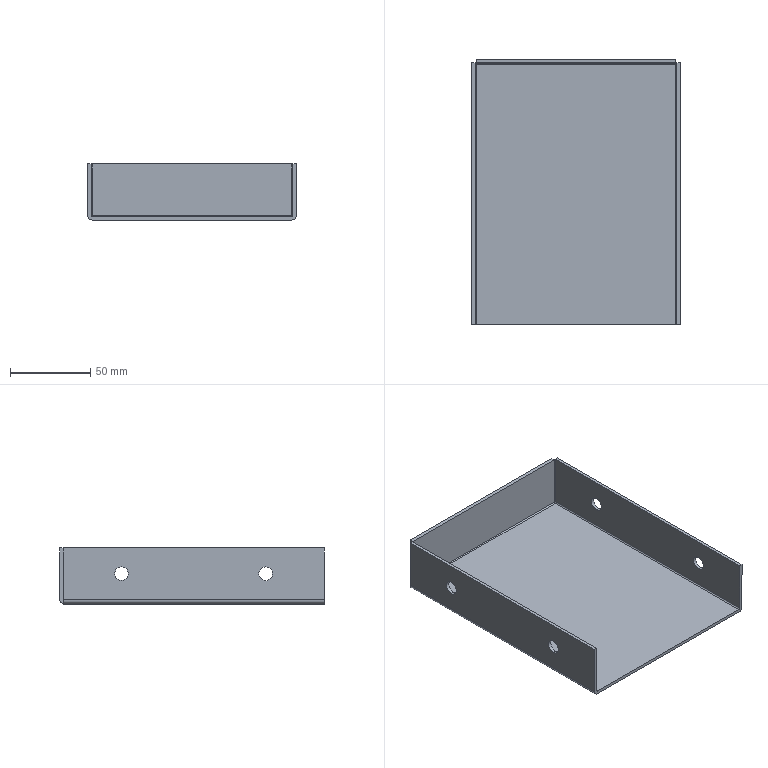Part | SolidWorks | features BaseBody 1 | 1 solid | 32 faces | box 130 x 165 x 35 mm | volume 71487 mm3 | plane 18 | cylinder 14 | commonest cylinder face diameters 8.5 x8 1.473 x3 5.473 x3
STEP:
#1=CARTESIAN_POINT('',(65.,45.,21.118));
#2=VERTEX_POINT('',#1);
#3=CARTESIAN_POINT('',(65.,45.,12.618));
#4=VERTEX_POINT('',#3);
#5=CARTESIAN_POINT('',(65.,45.,16.868));
#6=DIRECTION('',(1.,0.,0.));
#7=DIRECTION('',(0.,0.,1.));
#8=AXIS2_PLACEMENT_3D('',#5,#6,#7);
#9=CIRCLE('',#8,4.25);
#10=EDGE_CURVE('',#2,#4,#9,.T.);
#11=ORIENTED_EDGE('',*,*,#10,.T.);
#12=CARTESIAN_POINT('',(63.,45.,12.618));
#13=VERTEX_POINT('',#12);
#14=CARTESIAN_POINT('',(118.,45.,12.618));
#15=DIRECTION('',(-1.,0.,0.));
#16=VECTOR('',#15,1000.);
#17=LINE('',#14,#16);
#18=EDGE_CURVE('',#4,#13,#17,.T.);
#19=ORIENTED_EDGE('',*,*,#18,.T.);
#20=CARTESIAN_POINT('',(63.,45.,21.118));
#21=VERTEX_POINT('',#20);
#22=CARTESIAN_POINT('',(63.,45.,16.868));
#23=DIRECTION('',(1.,0.,0.));
#24=DIRECTION('',(0.,0.,1.));
#25=AXIS2_PLACEMENT_3D('',#22,#23,#24);
#26=CIRCLE('',#25,4.25);
#27=EDGE_CURVE('',#21,#13,#26,.T.);
#28=ORIENTED_EDGE('',*,*,#27,.F.);
#29=CARTESIAN_POINT('',(118.,45.,21.118));
#30=DIRECTION('',(-1.,0.,0.));
#31=VECTOR('',#30,1000.);
#32=LINE('',#29,#31);
#33=EDGE_CURVE('',#2,#21,#32,.T.);
#34=ORIENTED_EDGE('',*,*,#33,.F.);
#35=EDGE_LOOP('',(#11,#19,#28,#34));
#36=FACE_OUTER_BOUND('',#35,.T.);
#37=CARTESIAN_POINT('',(118.,45.,16.868));
#38=DIRECTION('',(-1.,0.,0.));
#39=DIRECTION('',(0.,0.,1.));
#40=AXIS2_PLACEMENT_3D('',#37,#38,#39);
#41=CYLINDRICAL_SURFACE('',#40,4.25);
#42=ADVANCED_FACE('',(#36),#41,.F.);
#43=CARTESIAN_POINT('',(65.,-45.,21.118));
#44=VERTEX_POINT('',#43);
#45=CARTESIAN_POINT('',(65.,-45.,12.618));
#46=VERTEX_POINT('',#45);
#47=CARTESIAN_POINT('',(65.,-45.,16.868));
#48=DIRECTION('',(1.,0.,0.));
#49=DIRECTION('',(0.,0.,1.));
#50=AXIS2_PLACEMENT_3D('',#47,#48,#49);
#51=CIRCLE('',#50,4.25);
#52=EDGE_CURVE('',#44,#46,#51,.T.);
#53=ORIENTED_EDGE('',*,*,#52,.T.);
#54=CARTESIAN_POINT('',(63.,-45.,12.618));
#55=VERTEX_POINT('',#54);
#56=CARTESIAN_POINT('',(118.,-45.,12.618));
#57=DIRECTION('',(-1.,0.,0.));
#58=VECTOR('',#57,1000.);
#59=LINE('',#56,#58);
#60=EDGE_CURVE('',#46,#55,#59,.T.);
#61=ORIENTED_EDGE('',*,*,#60,.T.);
#62=CARTESIAN_POINT('',(63.,-45.,21.118));
#63=VERTEX_POINT('',#62);
#64=CARTESIAN_POINT('',(63.,-45.,16.868));
#65=DIRECTION('',(1.,0.,0.));
#66=DIRECTION('',(0.,0.,1.));
#67=AXIS2_PLACEMENT_3D('',#64,#65,#66);
#68=CIRCLE('',#67,4.25);
#69=EDGE_CURVE('',#63,#55,#68,.T.);
#70=ORIENTED_EDGE('',*,*,#69,.F.);
#71=CARTESIAN_POINT('',(118.,-45.,21.118));
#72=DIRECTION('',(-1.,0.,0.));
#73=VECTOR('',#72,1000.);
#74=LINE('',#71,#73);
#75=EDGE_CURVE('',#44,#63,#74,.T.);
#76=ORIENTED_EDGE('',*,*,#75,.F.);
#77=EDGE_LOOP('',(#53,#61,#70,#76));
#78=FACE_OUTER_BOUND('',#77,.T.);
#79=CARTESIAN_POINT('',(118.,-45.,16.868));
#80=DIRECTION('',(-1.,0.,0.));
#81=DIRECTION('',(0.,0.,1.));
#82=AXIS2_PLACEMENT_3D('',#79,#80,#81);
#83=CYLINDRICAL_SURFACE('',#82,4.25);
#84=ADVANCED_FACE('',(#78),#83,.F.);
#85=CARTESIAN_POINT('',(-63.,45.,12.618));
#86=VERTEX_POINT('',#85);
#87=CARTESIAN_POINT('',(-63.,45.,21.118));
#88=VERTEX_POINT('',#87);
#89=CARTESIAN_POINT('',(-63.,45.,16.868));
#90=DIRECTION('',(-1.,0.,0.));
#91=DIRECTION('',(0.,0.,1.));
#92=AXIS2_PLACEMENT_3D('',#89,#90,#91);
#93=CIRCLE('',#92,4.25);
#94=EDGE_CURVE('',#86,#88,#93,.T.);
#95=ORIENTED_EDGE('',*,*,#94,.F.);
#96=CARTESIAN_POINT('',(-65.,45.,12.618));
#97=VERTEX_POINT('',#96);
#98=CARTESIAN_POINT('',(118.,45.,12.618));
#99=DIRECTION('',(-1.,0.,0.));
#100=VECTOR('',#99,1000.);
#101=LINE('',#98,#100);
#102=EDGE_CURVE('',#86,#97,#101,.T.);
#103=ORIENTED_EDGE('',*,*,#102,.T.);
#104=CARTESIAN_POINT('',(-65.,45.,21.118));
#105=VERTEX_POINT('',#104);
#106=CARTESIAN_POINT('',(-65.,45.,16.868));
#107=DIRECTION('',(-1.,0.,0.));
#108=DIRECTION('',(0.,0.,1.));
#109=AXIS2_PLACEMENT_3D('',#106,#107,#108);
#110=CIRCLE('',#109,4.25);
#111=EDGE_CURVE('',#97,#105,#110,.T.);
#112=ORIENTED_EDGE('',*,*,#111,.T.);
#113=CARTESIAN_POINT('',(118.,45.,21.118));
#114=DIRECTION('',(-1.,0.,0.));
#115=VECTOR('',#114,1000.);
#116=LINE('',#113,#115);
#117=EDGE_CURVE('',#88,#105,#116,.T.);
#118=ORIENTED_EDGE('',*,*,#117,.F.);
#119=EDGE_LOOP('',(#95,#103,#112,#118));
#120=FACE_OUTER_BOUND('',#119,.T.);
#121=CARTESIAN_POINT('',(118.,45.,16.868));
#122=DIRECTION('',(-1.,0.,0.));
#123=DIRECTION('',(0.,0.,1.));
#124=AXIS2_PLACEMENT_3D('',#121,#122,#123);
#125=CYLINDRICAL_SURFACE('',#124,4.25);
#126=ADVANCED_FACE('',(#120),#125,.F.);
#127=CARTESIAN_POINT('',(-63.,-45.,12.618));
#128=VERTEX_POINT('',#127);
#129=CARTESIAN_POINT('',(-63.,-45.,21.118));
#130=VERTEX_POINT('',#129);
#131=CARTESIAN_POINT('',(-63.,-45.,16.868));
#132=DIRECTION('',(-1.,0.,0.));
#133=DIRECTION('',(0.,0.,1.));
#134=AXIS2_PLACEMENT_3D('',#131,#132,#133);
#135=CIRCLE('',#134,4.25);
#136=EDGE_CURVE('',#128,#130,#135,.T.);
#137=ORIENTED_EDGE('',*,*,#136,.F.);
#138=CARTESIAN_POINT('',(-65.,-45.,12.618));
#139=VERTEX_POINT('',#138);
#140=CARTESIAN_POINT('',(118.,-45.,12.618));
#141=DIRECTION('',(-1.,0.,0.));
#142=VECTOR('',#141,1000.);
#143=LINE('',#140,#142);
#144=EDGE_CURVE('',#128,#139,#143,.T.);
#145=ORIENTED_EDGE('',*,*,#144,.T.);
#146=CARTESIAN_POINT('',(-65.,-45.,21.118));
#147=VERTEX_POINT('',#146);
#148=CARTESIAN_POINT('',(-65.,-45.,16.868));
#149=DIRECTION('',(-1.,0.,0.));
#150=DIRECTION('',(0.,0.,1.));
#151=AXIS2_PLACEMENT_3D('',#148,#149,#150);
#152=CIRCLE('',#151,4.25);
#153=EDGE_CURVE('',#139,#147,#152,.T.);
#154=ORIENTED_EDGE('',*,*,#153,.T.);
#155=CARTESIAN_POINT('',(118.,-45.,21.118));
#156=DIRECTION('',(-1.,0.,0.));
#157=VECTOR('',#156,1000.);
#158=LINE('',#155,#157);
#159=EDGE_CURVE('',#130,#147,#158,.T.);
#160=ORIENTED_EDGE('',*,*,#159,.F.);
#161=EDGE_LOOP('',(#137,#145,#154,#160));
#162=FACE_OUTER_BOUND('',#161,.T.);
#163=CARTESIAN_POINT('',(118.,-45.,16.868));
#164=DIRECTION('',(-1.,0.,0.));
#165=DIRECTION('',(0.,0.,1.));
#166=AXIS2_PLACEMENT_3D('',#163,#164,#165);
#167=CYLINDRICAL_SURFACE('',#166,4.25);
#168=ADVANCED_FACE('',(#162),#167,.F.);
#169=CARTESIAN_POINT('',(62.263,80.763,-2.));
#170=VERTEX_POINT('',#169);
#171=CARTESIAN_POINT('',(62.263,-81.5,-2.));
#172=VERTEX_POINT('',#171);
#173=CARTESIAN_POINT('',(62.263,0.,-2.));
#174=DIRECTION('',(0.,-1.,0.));
#175=VECTOR('',#174,1000.);
#176=LINE('',#173,#175);
#177=EDGE_CURVE('',#170,#172,#176,.T.);
#178=ORIENTED_EDGE('',*,*,#177,.T.);
#179=CARTESIAN_POINT('',(-62.263,-81.5,-2.));
#180=VERTEX_POINT('',#179);
#181=CARTESIAN_POINT('',(0.,-81.5,-2.));
#182=DIRECTION('',(-1.,0.,0.));
#183=VECTOR('',#182,1000.);
#184=LINE('',#181,#183);
#185=EDGE_CURVE('',#172,#180,#184,.T.);
#186=ORIENTED_EDGE('',*,*,#185,.T.);
#187=CARTESIAN_POINT('',(-62.263,80.763,-2.));
#188=VERTEX_POINT('',#187);
#189=CARTESIAN_POINT('',(-62.263,0.,-2.));
#190=DIRECTION('',(0.,1.,0.));
#191=VECTOR('',#190,1000.);
#192=LINE('',#189,#191);
#193=EDGE_CURVE('',#180,#188,#192,.T.);
#194=ORIENTED_EDGE('',*,*,#193,.T.);
#195=CARTESIAN_POINT('',(0.,80.763,-2.));
#196=DIRECTION('',(1.,0.,0.));
#197=VECTOR('',#196,1000.);
#198=LINE('',#195,#197);
#199=EDGE_CURVE('',#188,#170,#198,.T.);
#200=ORIENTED_EDGE('',*,*,#199,.T.);
#201=EDGE_LOOP('',(#178,#186,#194,#200));
#202=FACE_OUTER_BOUND('',#201,.T.);
#203=CARTESIAN_POINT('',(0.,0.,-2.));
#204=DIRECTION('',(0.,0.,-1.));
#205=DIRECTION('',(-1.,0.,0.));
#206=AXIS2_PLACEMENT_3D('',#203,#204,#205);
#207=PLANE('',#206);
#208=ADVANCED_FACE('',(#202),#207,.T.);
#209=ORIENTED_EDGE('',*,*,#185,.F.);
#210=CARTESIAN_POINT('',(65.,-81.5,0.7366));
#211=VERTEX_POINT('',#210);
#212=CARTESIAN_POINT('',(62.263,-81.5,0.7366));
#213=DIRECTION('',(0.,1.,0.));
#214=DIRECTION('',(0.,0.,1.));
#215=AXIS2_PLACEMENT_3D('',#212,#213,#214);
#216=CIRCLE('',#215,2.737);
#217=EDGE_CURVE('',#211,#172,#216,.T.);
#218=ORIENTED_EDGE('',*,*,#217,.F.);
#219=CARTESIAN_POINT('',(65.,-81.5,33.));
#220=VERTEX_POINT('',#219);
#221=CARTESIAN_POINT('',(65.,-81.5,0.));
#222=DIRECTION('',(0.,0.,1.));
#223=VECTOR('',#222,1000.);
#224=LINE('',#221,#223);
#225=EDGE_CURVE('',#211,#220,#224,.T.);
#226=ORIENTED_EDGE('',*,*,#225,.T.);
#227=CARTESIAN_POINT('',(63.,-81.5,33.));
#228=VERTEX_POINT('',#227);
#229=CARTESIAN_POINT('',(65.,-81.5,33.));
#230=DIRECTION('',(1.,0.,0.));
#231=VECTOR('',#230,1000.);
#232=LINE('',#229,#231);
#233=EDGE_CURVE('',#228,#220,#232,.T.);
#234=ORIENTED_EDGE('',*,*,#233,.F.);
#235=CARTESIAN_POINT('',(63.,-81.5,0.7366));
#236=VERTEX_POINT('',#235);
#237=CARTESIAN_POINT('',(63.,-81.5,0.));
#238=DIRECTION('',(0.,0.,1.));
#239=VECTOR('',#238,1000.);
#240=LINE('',#237,#239);
#241=EDGE_CURVE('',#236,#228,#240,.T.);
#242=ORIENTED_EDGE('',*,*,#241,.F.);
#243=CARTESIAN_POINT('',(62.263,-81.5,0.));
#244=VERTEX_POINT('',#243);
#245=CARTESIAN_POINT('',(62.263,-81.5,0.7366));
#246=DIRECTION('',(0.,1.,0.));
#247=DIRECTION('',(0.,0.,1.));
#248=AXIS2_PLACEMENT_3D('',#245,#246,#247);
#249=CIRCLE('',#248,0.7366);
#250=EDGE_CURVE('',#236,#244,#249,.T.);
#251=ORIENTED_EDGE('',*,*,#250,.T.);
#252=CARTESIAN_POINT('',(-62.263,-81.5,0.));
#253=VERTEX_POINT('',#252);
#254=CARTESIAN_POINT('',(-65.,-81.5,0.));
#255=DIRECTION('',(-1.,0.,0.));
#256=VECTOR('',#255,1000.);
#257=LINE('',#254,#256);
#258=EDGE_CURVE('',#244,#253,#257,.T.);
#259=ORIENTED_EDGE('',*,*,#258,.T.);
#260=CARTESIAN_POINT('',(-63.,-81.5,0.7366));
#261=VERTEX_POINT('',#260);
#262=CARTESIAN_POINT('',(-62.263,-81.5,0.7366));
#263=DIRECTION('',(0.,1.,0.));
#264=DIRECTION('',(0.,0.,-1.));
#265=AXIS2_PLACEMENT_3D('',#262,#263,#264);
#266=CIRCLE('',#265,0.7366);
#267=EDGE_CURVE('',#253,#261,#266,.T.);
#268=ORIENTED_EDGE('',*,*,#267,.T.);
#269=CARTESIAN_POINT('',(-63.,-81.5,33.));
#270=VERTEX_POINT('',#269);
#271=CARTESIAN_POINT('',(-63.,-81.5,33.));
#272=DIRECTION('',(0.,0.,-1.));
#273=VECTOR('',#272,1000.);
#274=LINE('',#271,#273);
#275=EDGE_CURVE('',#270,#261,#274,.T.);
#276=ORIENTED_EDGE('',*,*,#275,.F.);
#277=CARTESIAN_POINT('',(-65.,-81.5,33.));
#278=VERTEX_POINT('',#277);
#279=CARTESIAN_POINT('',(-65.,-81.5,33.));
#280=DIRECTION('',(1.,0.,0.));
#281=VECTOR('',#280,1000.);
#282=LINE('',#279,#281);
#283=EDGE_CURVE('',#278,#270,#282,.T.);
#284=ORIENTED_EDGE('',*,*,#283,.F.);
#285=CARTESIAN_POINT('',(-65.,-81.5,0.7366));
#286=VERTEX_POINT('',#285);
#287=CARTESIAN_POINT('',(-65.,-81.5,0.));
#288=DIRECTION('',(0.,0.,-1.));
#289=VECTOR('',#288,1000.);
#290=LINE('',#287,#289);
#291=EDGE_CURVE('',#278,#286,#290,.T.);
#292=ORIENTED_EDGE('',*,*,#291,.T.);
#293=CARTESIAN_POINT('',(-62.263,-81.5,0.7366));
#294=DIRECTION('',(0.,1.,0.));
#295=DIRECTION('',(0.,0.,-1.));
#296=AXIS2_PLACEMENT_3D('',#293,#294,#295);
#297=CIRCLE('',#296,2.737);
#298=EDGE_CURVE('',#180,#286,#297,.T.);
#299=ORIENTED_EDGE('',*,*,#298,.F.);
#300=EDGE_LOOP('',(#209,#218,#226,#234,#242,#251,#259,#268,#276,#284,#292,#299));
#301=FACE_OUTER_BOUND('',#300,.T.);
#302=CARTESIAN_POINT('',(-65.,-81.5,-2.));
#303=DIRECTION('',(0.,-1.,0.));
#304=DIRECTION('',(0.,0.,-1.));
#305=AXIS2_PLACEMENT_3D('',#302,#303,#304);
#306=PLANE('',#305);
#307=ADVANCED_FACE('',(#301),#306,.T.);
#308=ORIENTED_EDGE('',*,*,#217,.T.);
#309=ORIENTED_EDGE('',*,*,#177,.F.);
#310=CARTESIAN_POINT('',(62.263,81.5,-2.));
#311=VERTEX_POINT('',#310);
#312=CARTESIAN_POINT('',(62.263,81.5,-2.));
#313=DIRECTION('',(0.,1.,0.));
#314=VECTOR('',#313,1000.);
#315=LINE('',#312,#314);
#316=EDGE_CURVE('',#170,#311,#315,.T.);
#317=ORIENTED_EDGE('',*,*,#316,.T.);
#318=CARTESIAN_POINT('',(65.,81.5,0.7366));
#319=VERTEX_POINT('',#318);
#320=CARTESIAN_POINT('',(62.263,81.5,0.7366));
#321=DIRECTION('',(0.,-1.,0.));
#322=DIRECTION('',(0.,0.,1.));
#323=AXIS2_PLACEMENT_3D('',#320,#321,#322);
#324=CIRCLE('',#323,2.737);
#325=EDGE_CURVE('',#311,#319,#324,.T.);
#326=ORIENTED_EDGE('',*,*,#325,.T.);
#327=CARTESIAN_POINT('',(65.,81.5,0.7366));
#328=DIRECTION('',(0.,-1.,0.));
#329=VECTOR('',#328,1000.);
#330=LINE('',#327,#329);
#331=EDGE_CURVE('',#319,#211,#330,.T.);
#332=ORIENTED_EDGE('',*,*,#331,.T.);
#333=EDGE_LOOP('',(#308,#309,#317,#326,#332));
#334=FACE_OUTER_BOUND('',#333,.T.);
#335=CARTESIAN_POINT('',(62.263,81.5,0.7366));
#336=DIRECTION('',(0.,1.,0.));
#337=DIRECTION('',(0.,0.,1.));
#338=AXIS2_PLACEMENT_3D('',#335,#336,#337);
#339=CYLINDRICAL_SURFACE('',#338,2.737);
#340=ADVANCED_FACE('',(#334),#339,.T.);
#341=CARTESIAN_POINT('',(62.263,83.5,0.7366));
#342=VERTEX_POINT('',#341);
#343=CARTESIAN_POINT('',(62.263,81.5,-1.899));
#344=VERTEX_POINT('',#343);
#345=CARTESIAN_POINT('',(62.263,80.763,0.7366));
#346=DIRECTION('',(-1.,0.,0.));
#347=DIRECTION('',(0.,0.,1.));
#348=AXIS2_PLACEMENT_3D('',#345,#346,#347);
#349=CIRCLE('',#348,2.737);
#350=EDGE_CURVE('',#342,#344,#349,.T.);
#351=ORIENTED_EDGE('',*,*,#350,.T.);
#352=CARTESIAN_POINT('',(62.263,80.763,0.7366));
#353=DIRECTION('',(-1.,0.,0.));
#354=DIRECTION('',(0.,0.,1.));
#355=AXIS2_PLACEMENT_3D('',#352,#353,#354);
#356=CIRCLE('',#355,2.737);
#357=EDGE_CURVE('',#344,#170,#356,.T.);
#358=ORIENTED_EDGE('',*,*,#357,.T.);
#359=ORIENTED_EDGE('',*,*,#199,.F.);
#360=CARTESIAN_POINT('',(-62.263,81.5,-1.899));
#361=VERTEX_POINT('',#360);
#362=CARTESIAN_POINT('',(-62.263,80.763,0.7366));
#363=DIRECTION('',(1.,0.,0.));
#364=DIRECTION('',(0.,0.,1.));
#365=AXIS2_PLACEMENT_3D('',#362,#363,#364);
#366=CIRCLE('',#365,2.737);
#367=EDGE_CURVE('',#188,#361,#366,.T.);
#368=ORIENTED_EDGE('',*,*,#367,.T.);
#369=CARTESIAN_POINT('',(-62.263,83.5,0.7366));
#370=VERTEX_POINT('',#369);
#371=CARTESIAN_POINT('',(-62.263,80.763,0.7366));
#372=DIRECTION('',(1.,0.,0.));
#373=DIRECTION('',(0.,0.,1.));
#374=AXIS2_PLACEMENT_3D('',#371,#372,#373);
#375=CIRCLE('',#374,2.737);
#376=EDGE_CURVE('',#361,#370,#375,.T.);
#377=ORIENTED_EDGE('',*,*,#376,.T.);
#378=CARTESIAN_POINT('',(-62.263,83.5,0.7366));
#379=DIRECTION('',(1.,0.,0.));
#380=VECTOR('',#379,1000.);
#381=LINE('',#378,#380);
#382=EDGE_CURVE('',#370,#342,#381,.T.);
#383=ORIENTED_EDGE('',*,*,#382,.T.);
#384=EDGE_LOOP('',(#351,#358,#359,#368,#377,#383));
#385=FACE_OUTER_BOUND('',#384,.T.);
#386=CARTESIAN_POINT('',(-62.263,80.763,0.7366));
#387=DIRECTION('',(-1.,0.,0.));
#388=DIRECTION('',(0.,0.,1.));
#389=AXIS2_PLACEMENT_3D('',#386,#387,#388);
#390=CYLINDRICAL_SURFACE('',#389,2.737);
#391=ADVANCED_FACE('',(#385),#390,.T.);
#392=CARTESIAN_POINT('',(-65.,81.5,0.7366));
#393=VERTEX_POINT('',#392);
#394=CARTESIAN_POINT('',(-62.263,81.5,-2.));
#395=VERTEX_POINT('',#394);
#396=CARTESIAN_POINT('',(-62.263,81.5,0.7366));
#397=DIRECTION('',(0.,-1.,0.));
#398=DIRECTION('',(0.,0.,-1.));
#399=AXIS2_PLACEMENT_3D('',#396,#397,#398);
#400=CIRCLE('',#399,2.737);
#401=EDGE_CURVE('',#393,#395,#400,.T.);
#402=ORIENTED_EDGE('',*,*,#401,.T.);
#403=CARTESIAN_POINT('',(-62.263,81.5,-2.));
#404=DIRECTION('',(0.,-1.,0.));
#405=VECTOR('',#404,1000.);
#406=LINE('',#403,#405);
#407=EDGE_CURVE('',#395,#188,#406,.T.);
#408=ORIENTED_EDGE('',*,*,#407,.T.);
#409=ORIENTED_EDGE('',*,*,#193,.F.);
#410=ORIENTED_EDGE('',*,*,#298,.T.);
#411=CARTESIAN_POINT('',(-65.,-81.5,0.7366));
#412=DIRECTION('',(0.,1.,0.));
#413=VECTOR('',#412,1000.);
#414=LINE('',#411,#413);
#415=EDGE_CURVE('',#286,#393,#414,.T.);
#416=ORIENTED_EDGE('',*,*,#415,.T.);
#417=EDGE_LOOP('',(#402,#408,#409,#410,#416));
#418=FACE_OUTER_BOUND('',#417,.T.);
#419=CARTESIAN_POINT('',(-62.263,-81.5,0.7366));
#420=DIRECTION('',(0.,-1.,0.));
#421=DIRECTION('',(0.,0.,-1.));
#422=AXIS2_PLACEMENT_3D('',#419,#420,#421);
#423=CYLINDRICAL_SURFACE('',#422,2.737);
#424=ADVANCED_FACE('',(#418),#423,.T.);
#425=CARTESIAN_POINT('',(-62.263,80.763,0.));
#426=VERTEX_POINT('',#425);
#427=CARTESIAN_POINT('',(-62.263,0.,0.));
#428=DIRECTION('',(0.,1.,0.));
#429=VECTOR('',#428,1000.);
#430=LINE('',#427,#429);
#431=EDGE_CURVE('',#253,#426,#430,.T.);
#432=ORIENTED_EDGE('',*,*,#431,.F.);
#433=ORIENTED_EDGE('',*,*,#258,.F.);
#434=CARTESIAN_POINT('',(62.263,80.763,0.));
#435=VERTEX_POINT('',#434);
#436=CARTESIAN_POINT('',(62.263,0.,0.));
#437=DIRECTION('',(0.,-1.,0.));
#438=VECTOR('',#437,1000.);
#439=LINE('',#436,#438);
#440=EDGE_CURVE('',#435,#244,#439,.T.);
#441=ORIENTED_EDGE('',*,*,#440,.F.);
#442=CARTESIAN_POINT('',(0.,80.763,0.));
#443=DIRECTION('',(1.,0.,0.));
#444=VECTOR('',#443,1000.);
#445=LINE('',#442,#444);
#446=EDGE_CURVE('',#426,#435,#445,.T.);
#447=ORIENTED_EDGE('',*,*,#446,.F.);
#448=EDGE_LOOP('',(#432,#433,#441,#447));
#449=FACE_OUTER_BOUND('',#448,.T.);
#450=CARTESIAN_POINT('',(0.,0.,0.));
#451=DIRECTION('',(0.,0.,-1.));
#452=DIRECTION('',(-1.,0.,0.));
#453=AXIS2_PLACEMENT_3D('',#450,#451,#452);
#454=PLANE('',#453);
#455=ADVANCED_FACE('',(#449),#454,.F.);
#456=CARTESIAN_POINT('',(65.,81.5,33.));
#457=VERTEX_POINT('',#456);
#458=CARTESIAN_POINT('',(65.,81.5,0.));
#459=DIRECTION('',(0.,0.,-1.));
#460=VECTOR('',#459,1000.);
#461=LINE('',#458,#460);
#462=EDGE_CURVE('',#457,#319,#461,.T.);
#463=ORIENTED_EDGE('',*,*,#462,.F.);
#464=CARTESIAN_POINT('',(65.,0.,33.));
#465=DIRECTION('',(0.,1.,0.));
#466=VECTOR('',#465,1000.);
#467=LINE('',#464,#466);
#468=EDGE_CURVE('',#220,#457,#467,.T.);
#469=ORIENTED_EDGE('',*,*,#468,.F.);
#470=ORIENTED_EDGE('',*,*,#225,.F.);
#471=ORIENTED_EDGE('',*,*,#331,.F.);
#472=EDGE_LOOP('',(#463,#469,#470,#471));
#473=FACE_OUTER_BOUND('',#472,.T.);
#474=ORIENTED_EDGE('',*,*,#10,.F.);
#475=CARTESIAN_POINT('',(65.,45.,16.868));
#476=DIRECTION('',(1.,0.,0.));
#477=DIRECTION('',(0.,0.,1.));
#478=AXIS2_PLACEMENT_3D('',#475,#476,#477);
#479=CIRCLE('',#478,4.25);
#480=EDGE_CURVE('',#4,#2,#479,.T.);
#481=ORIENTED_EDGE('',*,*,#480,.F.);
#482=EDGE_LOOP('',(#474,#481));
#483=FACE_BOUND('',#482,.T.);
#484=ORIENTED_EDGE('',*,*,#52,.F.);
#485=CARTESIAN_POINT('',(65.,-45.,16.868));
#486=DIRECTION('',(1.,0.,0.));
#487=DIRECTION('',(0.,0.,1.));
#488=AXIS2_PLACEMENT_3D('',#485,#486,#487);
#489=CIRCLE('',#488,4.25);
#490=EDGE_CURVE('',#46,#44,#489,.T.);
#491=ORIENTED_EDGE('',*,*,#490,.F.);
#492=EDGE_LOOP('',(#484,#491));
#493=FACE_BOUND('',#492,.T.);
#494=CARTESIAN_POINT('',(65.,0.,0.));
#495=DIRECTION('',(-1.,0.,0.));
#496=DIRECTION('',(0.,0.,1.));
#497=AXIS2_PLACEMENT_3D('',#494,#495,#496);
#498=PLANE('',#497);
#499=ADVANCED_FACE('',(#473,#483,#493),#498,.F.);
#500=CARTESIAN_POINT('',(63.,81.5,0.7366));
#501=VERTEX_POINT('',#500);
#502=CARTESIAN_POINT('',(62.263,81.5,0.));
#503=VERTEX_POINT('',#502);
#504=CARTESIAN_POINT('',(62.263,81.5,0.7366));
#505=DIRECTION('',(0.,1.,0.));
#506=DIRECTION('',(0.,0.,1.));
#507=AXIS2_PLACEMENT_3D('',#504,#505,#506);
#508=CIRCLE('',#507,0.7366);
#509=EDGE_CURVE('',#501,#503,#508,.T.);
#510=ORIENTED_EDGE('',*,*,#509,.F.);
#511=CARTESIAN_POINT('',(63.,81.5,33.));
#512=VERTEX_POINT('',#511);
#513=CARTESIAN_POINT('',(63.,81.5,33.));
#514=DIRECTION('',(0.,0.,-1.));
#515=VECTOR('',#514,1000.);
#516=LINE('',#513,#515);
#517=EDGE_CURVE('',#512,#501,#516,.T.);
#518=ORIENTED_EDGE('',*,*,#517,.F.);
#519=CARTESIAN_POINT('',(65.,81.5,33.));
#520=DIRECTION('',(-1.,0.,0.));
#521=VECTOR('',#520,1000.);
#522=LINE('',#519,#521);
#523=EDGE_CURVE('',#457,#512,#522,.T.);
#524=ORIENTED_EDGE('',*,*,#523,.F.);
#525=ORIENTED_EDGE('',*,*,#462,.T.);
#526=ORIENTED_EDGE('',*,*,#325,.F.);
#527=CARTESIAN_POINT('',(62.263,81.5,0.7366));
#528=DIRECTION('',(0.,0.,-1.));
#529=VECTOR('',#528,1000.);
#530=LINE('',#527,#529);
#531=EDGE_CURVE('',#344,#311,#530,.T.);
#532=ORIENTED_EDGE('',*,*,#531,.F.);
#533=CARTESIAN_POINT('',(62.263,81.5,0.7366));
#534=DIRECTION('',(0.,0.,-1.));
#535=VECTOR('',#534,1000.);
#536=LINE('',#533,#535);
#537=EDGE_CURVE('',#503,#344,#536,.T.);
#538=ORIENTED_EDGE('',*,*,#537,.F.);
#539=EDGE_LOOP('',(#510,#518,#524,#525,#526,#532,#538));
#540=FACE_OUTER_BOUND('',#539,.T.);
#541=CARTESIAN_POINT('',(62.263,81.5,0.7366));
#542=DIRECTION('',(0.,-1.,0.));
#543=DIRECTION('',(0.,0.,-1.));
#544=AXIS2_PLACEMENT_3D('',#541,#542,#543);
#545=PLANE('',#544);
#546=ADVANCED_FACE('',(#540),#545,.F.);
#547=ORIENTED_EDGE('',*,*,#357,.F.);
#548=ORIENTED_EDGE('',*,*,#531,.T.);
#549=ORIENTED_EDGE('',*,*,#316,.F.);
#550=EDGE_LOOP('',(#547,#548,#549));
#551=FACE_OUTER_BOUND('',#550,.T.);
#552=CARTESIAN_POINT('',(62.263,80.763,0.));
#553=DIRECTION('',(-1.,0.,0.));
#554=DIRECTION('',(0.,0.,1.));
#555=AXIS2_PLACEMENT_3D('',#552,#553,#554);
#556=PLANE('',#555);
#557=ADVANCED_FACE('',(#551),#556,.T.);
#558=ORIENTED_EDGE('',*,*,#350,.F.);
#559=CARTESIAN_POINT('',(62.263,83.5,33.));
#560=VERTEX_POINT('',#559);
#561=CARTESIAN_POINT('',(62.263,83.5,0.));
#562=DIRECTION('',(0.,0.,1.));
#563=VECTOR('',#562,1000.);
#564=LINE('',#561,#563);
#565=EDGE_CURVE('',#342,#560,#564,.T.);
#566=ORIENTED_EDGE('',*,*,#565,.T.);
#567=CARTESIAN_POINT('',(62.263,81.5,33.));
#568=VERTEX_POINT('',#567);
#569=CARTESIAN_POINT('',(62.263,83.5,33.));
#570=DIRECTION('',(0.,1.,0.));
#571=VECTOR('',#570,1000.);
#572=LINE('',#569,#571);
#573=EDGE_CURVE('',#568,#560,#572,.T.);
#574=ORIENTED_EDGE('',*,*,#573,.F.);
#575=CARTESIAN_POINT('',(62.263,81.5,0.7366));
#576=VERTEX_POINT('',#575);
#577=CARTESIAN_POINT('',(62.263,81.5,0.));
#578=DIRECTION('',(0.,0.,1.));
#579=VECTOR('',#578,1000.);
#580=LINE('',#577,#579);
#581=EDGE_CURVE('',#576,#568,#580,.T.);
#582=ORIENTED_EDGE('',*,*,#581,.F.);
#583=CARTESIAN_POINT('',(62.263,80.763,0.7366));
#584=DIRECTION('',(-1.,0.,0.));
#585=DIRECTION('',(0.,0.,1.));
#586=AXIS2_PLACEMENT_3D('',#583,#584,#585);
#587=CIRCLE('',#586,0.7366);
#588=EDGE_CURVE('',#576,#435,#587,.T.);
#589=ORIENTED_EDGE('',*,*,#588,.T.);
#590=CARTESIAN_POINT('',(62.263,80.763,0.));
#591=DIRECTION('',(0.,1.,0.));
#592=VECTOR('',#591,1000.);
#593=LINE('',#590,#592);
#594=EDGE_CURVE('',#435,#503,#593,.T.);
#595=ORIENTED_EDGE('',*,*,#594,.T.);
#596=ORIENTED_EDGE('',*,*,#537,.T.);
#597=EDGE_LOOP('',(#558,#566,#574,#582,#589,#595,#596));
#598=FACE_OUTER_BOUND('',#597,.T.);
#599=CARTESIAN_POINT('',(62.263,80.763,0.7366));
#600=DIRECTION('',(1.,0.,0.));
#601=DIRECTION('',(0.,0.,-1.));
#602=AXIS2_PLACEMENT_3D('',#599,#600,#601);
#603=PLANE('',#602);
#604=ADVANCED_FACE('',(#598),#603,.T.);
#605=CARTESIAN_POINT('',(-62.263,83.5,33.));
#606=VERTEX_POINT('',#605);
#607=CARTESIAN_POINT('',(-62.263,83.5,0.));
#608=DIRECTION('',(0.,0.,-1.));
#609=VECTOR('',#608,1000.);
#610=LINE('',#607,#609);
#611=EDGE_CURVE('',#606,#370,#610,.T.);
#612=ORIENTED_EDGE('',*,*,#611,.F.);
#613=CARTESIAN_POINT('',(0.,83.5,33.));
#614=DIRECTION('',(-1.,0.,0.));
#615=VECTOR('',#614,1000.);
#616=LINE('',#613,#615);
#617=EDGE_CURVE('',#560,#606,#616,.T.);
#618=ORIENTED_EDGE('',*,*,#617,.F.);
#619=ORIENTED_EDGE('',*,*,#565,.F.);
#620=ORIENTED_EDGE('',*,*,#382,.F.);
#621=EDGE_LOOP('',(#612,#618,#619,#620));
#622=FACE_OUTER_BOUND('',#621,.T.);
#623=CARTESIAN_POINT('',(0.,83.5,0.));
#624=DIRECTION('',(0.,-1.,0.));
#625=DIRECTION('',(0.,0.,-1.));
#626=AXIS2_PLACEMENT_3D('',#623,#624,#625);
#627=PLANE('',#626);
#628=ADVANCED_FACE('',(#622),#627,.F.);
#629=CARTESIAN_POINT('',(-62.263,81.5,0.));
#630=VERTEX_POINT('',#629);
#631=CARTESIAN_POINT('',(-62.263,80.763,0.));
#632=DIRECTION('',(0.,1.,0.));
#633=VECTOR('',#632,1000.);
#634=LINE('',#631,#633);
#635=EDGE_CURVE('',#426,#630,#634,.T.);
#636=ORIENTED_EDGE('',*,*,#635,.F.);
#637=CARTESIAN_POINT('',(-62.263,81.5,0.7366));
#638=VERTEX_POINT('',#637);
#639=CARTESIAN_POINT('',(-62.263,80.763,0.7366));
#640=DIRECTION('',(-1.,0.,0.));
#641=DIRECTION('',(0.,0.,1.));
#642=AXIS2_PLACEMENT_3D('',#639,#640,#641);
#643=CIRCLE('',#642,0.7366);
#644=EDGE_CURVE('',#638,#426,#643,.T.);
#645=ORIENTED_EDGE('',*,*,#644,.F.);
#646=CARTESIAN_POINT('',(-62.263,81.5,33.));
#647=VERTEX_POINT('',#646);
#648=CARTESIAN_POINT('',(-62.263,81.5,33.));
#649=DIRECTION('',(0.,0.,-1.));
#650=VECTOR('',#649,1000.);
#651=LINE('',#648,#650);
#652=EDGE_CURVE('',#647,#638,#651,.T.);
#653=ORIENTED_EDGE('',*,*,#652,.F.);
#654=CARTESIAN_POINT('',(-62.263,83.5,33.));
#655=DIRECTION('',(0.,-1.,0.));
#656=VECTOR('',#655,1000.);
#657=LINE('',#654,#656);
#658=EDGE_CURVE('',#606,#647,#657,.T.);
#659=ORIENTED_EDGE('',*,*,#658,.F.);
#660=ORIENTED_EDGE('',*,*,#611,.T.);
#661=ORIENTED_EDGE('',*,*,#376,.F.);
#662=CARTESIAN_POINT('',(-62.263,81.5,0.7366));
#663=DIRECTION('',(0.,0.,-1.));
#664=VECTOR('',#663,1000.);
#665=LINE('',#662,#664);
#666=EDGE_CURVE('',#630,#361,#665,.T.);
#667=ORIENTED_EDGE('',*,*,#666,.F.);
#668=EDGE_LOOP('',(#636,#645,#653,#659,#660,#661,#667));
#669=FACE_OUTER_BOUND('',#668,.T.);
#670=CARTESIAN_POINT('',(-62.263,80.763,0.7366));
#671=DIRECTION('',(1.,0.,0.));
#672=DIRECTION('',(0.,0.,-1.));
#673=AXIS2_PLACEMENT_3D('',#670,#671,#672);
#674=PLANE('',#673);
#675=ADVANCED_FACE('',(#669),#674,.F.);
#676=ORIENTED_EDGE('',*,*,#367,.F.);
#677=ORIENTED_EDGE('',*,*,#407,.F.);
#678=CARTESIAN_POINT('',(-62.263,81.5,0.));
#679=DIRECTION('',(0.,0.,1.));
#680=VECTOR('',#679,1000.);
#681=LINE('',#678,#680);
#682=EDGE_CURVE('',#395,#361,#681,.T.);
#683=ORIENTED_EDGE('',*,*,#682,.T.);
#684=EDGE_LOOP('',(#676,#677,#683));
#685=FACE_OUTER_BOUND('',#684,.T.);
#686=CARTESIAN_POINT('',(-62.263,81.5,0.));
#687=DIRECTION('',(1.,0.,0.));
#688=DIRECTION('',(0.,1.,0.));
#689=AXIS2_PLACEMENT_3D('',#686,#687,#688);
#690=PLANE('',#689);
#691=ADVANCED_FACE('',(#685),#690,.T.);
#692=ORIENTED_EDGE('',*,*,#682,.F.);
#693=ORIENTED_EDGE('',*,*,#401,.F.);
#694=CARTESIAN_POINT('',(-65.,81.5,33.));
#695=VERTEX_POINT('',#694);
#696=CARTESIAN_POINT('',(-65.,81.5,0.));
#697=DIRECTION('',(0.,0.,1.));
#698=VECTOR('',#697,1000.);
#699=LINE('',#696,#698);
#700=EDGE_CURVE('',#393,#695,#699,.T.);
#701=ORIENTED_EDGE('',*,*,#700,.T.);
#702=CARTESIAN_POINT('',(-63.,81.5,33.));
#703=VERTEX_POINT('',#702);
#704=CARTESIAN_POINT('',(-65.,81.5,33.));
#705=DIRECTION('',(-1.,0.,0.));
#706=VECTOR('',#705,1000.);
#707=LINE('',#704,#706);
#708=EDGE_CURVE('',#703,#695,#707,.T.);
#709=ORIENTED_EDGE('',*,*,#708,.F.);
#710=CARTESIAN_POINT('',(-63.,81.5,0.7366));
#711=VERTEX_POINT('',#710);
#712=CARTESIAN_POINT('',(-63.,81.5,0.));
#713=DIRECTION('',(0.,0.,1.));
#714=VECTOR('',#713,1000.);
#715=LINE('',#712,#714);
#716=EDGE_CURVE('',#711,#703,#715,.T.);
#717=ORIENTED_EDGE('',*,*,#716,.F.);
#718=CARTESIAN_POINT('',(-62.263,81.5,0.7366));
#719=DIRECTION('',(0.,-1.,0.));
#720=DIRECTION('',(0.,0.,-1.));
#721=AXIS2_PLACEMENT_3D('',#718,#719,#720);
#722=CIRCLE('',#721,0.7366);
#723=EDGE_CURVE('',#711,#630,#722,.T.);
#724=ORIENTED_EDGE('',*,*,#723,.T.);
#725=ORIENTED_EDGE('',*,*,#666,.T.);
#726=EDGE_LOOP('',(#692,#693,#701,#709,#717,#724,#725));
#727=FACE_OUTER_BOUND('',#726,.T.);
#728=CARTESIAN_POINT('',(-62.263,81.5,0.7366));
#729=DIRECTION('',(0.,1.,0.));
#730=DIRECTION('',(0.,0.,1.));
#731=AXIS2_PLACEMENT_3D('',#728,#729,#730);
#732=PLANE('',#731);
#733=ADVANCED_FACE('',(#727),#732,.T.);
#734=ORIENTED_EDGE('',*,*,#291,.F.);
#735=CARTESIAN_POINT('',(-65.,0.,33.));
#736=DIRECTION('',(0.,-1.,0.));
#737=VECTOR('',#736,1000.);
#738=LINE('',#735,#737);
#739=EDGE_CURVE('',#695,#278,#738,.T.);
#740=ORIENTED_EDGE('',*,*,#739,.F.);
#741=ORIENTED_EDGE('',*,*,#700,.F.);
#742=ORIENTED_EDGE('',*,*,#415,.F.);
#743=EDGE_LOOP('',(#734,#740,#741,#742));
#744=FACE_OUTER_BOUND('',#743,.T.);
#745=CARTESIAN_POINT('',(-65.,45.,16.868));
#746=DIRECTION('',(-1.,0.,0.));
#747=DIRECTION('',(0.,0.,1.));
#748=AXIS2_PLACEMENT_3D('',#745,#746,#747);
#749=CIRCLE('',#748,4.25);
#750=EDGE_CURVE('',#105,#97,#749,.T.);
#751=ORIENTED_EDGE('',*,*,#750,.F.);
#752=ORIENTED_EDGE('',*,*,#111,.F.);
#753=EDGE_LOOP('',(#751,#752));
#754=FACE_BOUND('',#753,.T.);
#755=CARTESIAN_POINT('',(-65.,-45.,16.868));
#756=DIRECTION('',(-1.,0.,0.));
#757=DIRECTION('',(0.,0.,1.));
#758=AXIS2_PLACEMENT_3D('',#755,#756,#757);
#759=CIRCLE('',#758,4.25);
#760=EDGE_CURVE('',#147,#139,#759,.T.);
#761=ORIENTED_EDGE('',*,*,#760,.F.);
#762=ORIENTED_EDGE('',*,*,#153,.F.);
#763=EDGE_LOOP('',(#761,#762));
#764=FACE_BOUND('',#763,.T.);
#765=CARTESIAN_POINT('',(-65.,0.,0.));
#766=DIRECTION('',(1.,0.,0.));
#767=DIRECTION('',(0.,0.,-1.));
#768=AXIS2_PLACEMENT_3D('',#765,#766,#767);
#769=PLANE('',#768);
#770=ADVANCED_FACE('',(#744,#754,#764),#769,.F.);
#771=ORIENTED_EDGE('',*,*,#588,.F.);
#772=CARTESIAN_POINT('',(-62.263,81.5,0.7366));
#773=DIRECTION('',(1.,0.,0.));
#774=VECTOR('',#773,1000.);
#775=LINE('',#772,#774);
#776=EDGE_CURVE('',#638,#576,#775,.T.);
#777=ORIENTED_EDGE('',*,*,#776,.F.);
#778=ORIENTED_EDGE('',*,*,#644,.T.);
#779=ORIENTED_EDGE('',*,*,#446,.T.);
#780=EDGE_LOOP('',(#771,#777,#778,#779));
#781=FACE_OUTER_BOUND('',#780,.T.);
#782=CARTESIAN_POINT('',(-62.263,80.763,0.7366));
#783=DIRECTION('',(-1.,0.,0.));
#784=DIRECTION('',(0.,0.,1.));
#785=AXIS2_PLACEMENT_3D('',#782,#783,#784);
#786=CYLINDRICAL_SURFACE('',#785,0.7366);
#787=ADVANCED_FACE('',(#781),#786,.F.);
#788=ORIENTED_EDGE('',*,*,#635,.T.);
#789=ORIENTED_EDGE('',*,*,#723,.F.);
#790=CARTESIAN_POINT('',(-63.,-81.5,0.7366));
#791=DIRECTION('',(0.,1.,0.));
#792=VECTOR('',#791,1000.);
#793=LINE('',#790,#792);
#794=EDGE_CURVE('',#261,#711,#793,.T.);
#795=ORIENTED_EDGE('',*,*,#794,.F.);
#796=ORIENTED_EDGE('',*,*,#267,.F.);
#797=ORIENTED_EDGE('',*,*,#431,.T.);
#798=EDGE_LOOP('',(#788,#789,#795,#796,#797));
#799=FACE_OUTER_BOUND('',#798,.T.);
#800=CARTESIAN_POINT('',(-62.263,-81.5,0.7366));
#801=DIRECTION('',(0.,-1.,0.));
#802=DIRECTION('',(0.,0.,-1.));
#803=AXIS2_PLACEMENT_3D('',#800,#801,#802);
#804=CYLINDRICAL_SURFACE('',#803,0.7366);
#805=ADVANCED_FACE('',(#799),#804,.F.);
#806=ORIENTED_EDGE('',*,*,#440,.T.);
#807=ORIENTED_EDGE('',*,*,#250,.F.);
#808=CARTESIAN_POINT('',(63.,81.5,0.7366));
#809=DIRECTION('',(0.,-1.,0.));
#810=VECTOR('',#809,1000.);
#811=LINE('',#808,#810);
#812=EDGE_CURVE('',#501,#236,#811,.T.);
#813=ORIENTED_EDGE('',*,*,#812,.F.);
#814=ORIENTED_EDGE('',*,*,#509,.T.);
#815=ORIENTED_EDGE('',*,*,#594,.F.);
#816=EDGE_LOOP('',(#806,#807,#813,#814,#815));
#817=FACE_OUTER_BOUND('',#816,.T.);
#818=CARTESIAN_POINT('',(62.263,81.5,0.7366));
#819=DIRECTION('',(0.,1.,0.));
#820=DIRECTION('',(0.,0.,1.));
#821=AXIS2_PLACEMENT_3D('',#818,#819,#820);
#822=CYLINDRICAL_SURFACE('',#821,0.7366);
#823=ADVANCED_FACE('',(#817),#822,.F.);
#824=ORIENTED_EDGE('',*,*,#233,.T.);
#825=ORIENTED_EDGE('',*,*,#468,.T.);
#826=ORIENTED_EDGE('',*,*,#523,.T.);
#827=CARTESIAN_POINT('',(63.,-81.5,33.));
#828=DIRECTION('',(0.,1.,0.));
#829=VECTOR('',#828,1000.);
#830=LINE('',#827,#829);
#831=EDGE_CURVE('',#228,#512,#830,.T.);
#832=ORIENTED_EDGE('',*,*,#831,.F.);
#833=EDGE_LOOP('',(#824,#825,#826,#832));
#834=FACE_OUTER_BOUND('',#833,.T.);
#835=CARTESIAN_POINT('',(65.,-81.5,33.));
#836=DIRECTION('',(0.,0.,-1.));
#837=DIRECTION('',(-1.,0.,0.));
#838=AXIS2_PLACEMENT_3D('',#835,#836,#837);
#839=PLANE('',#838);
#840=ADVANCED_FACE('',(#834),#839,.F.);
#841=ORIENTED_EDGE('',*,*,#18,.F.);
#842=ORIENTED_EDGE('',*,*,#480,.T.);
#843=ORIENTED_EDGE('',*,*,#33,.T.);
#844=CARTESIAN_POINT('',(63.,45.,16.868));
#845=DIRECTION('',(1.,0.,0.));
#846=DIRECTION('',(0.,0.,1.));
#847=AXIS2_PLACEMENT_3D('',#844,#845,#846);
#848=CIRCLE('',#847,4.25);
#849=EDGE_CURVE('',#13,#21,#848,.T.);
#850=ORIENTED_EDGE('',*,*,#849,.F.);
#851=EDGE_LOOP('',(#841,#842,#843,#850));
#852=FACE_OUTER_BOUND('',#851,.T.);
#853=CARTESIAN_POINT('',(118.,45.,16.868));
#854=DIRECTION('',(-1.,0.,0.));
#855=DIRECTION('',(0.,0.,1.));
#856=AXIS2_PLACEMENT_3D('',#853,#854,#855);
#857=CYLINDRICAL_SURFACE('',#856,4.25);
#858=ADVANCED_FACE('',(#852),#857,.F.);
#859=ORIENTED_EDGE('',*,*,#60,.F.);
#860=ORIENTED_EDGE('',*,*,#490,.T.);
#861=ORIENTED_EDGE('',*,*,#75,.T.);
#862=CARTESIAN_POINT('',(63.,-45.,16.868));
#863=DIRECTION('',(1.,0.,0.));
#864=DIRECTION('',(0.,0.,1.));
#865=AXIS2_PLACEMENT_3D('',#862,#863,#864);
#866=CIRCLE('',#865,4.25);
#867=EDGE_CURVE('',#55,#63,#866,.T.);
#868=ORIENTED_EDGE('',*,*,#867,.F.);
#869=EDGE_LOOP('',(#859,#860,#861,#868));
#870=FACE_OUTER_BOUND('',#869,.T.);
#871=CARTESIAN_POINT('',(118.,-45.,16.868));
#872=DIRECTION('',(-1.,0.,0.));
#873=DIRECTION('',(0.,0.,1.));
#874=AXIS2_PLACEMENT_3D('',#871,#872,#873);
#875=CYLINDRICAL_SURFACE('',#874,4.25);
#876=ADVANCED_FACE('',(#870),#875,.F.);
#877=ORIENTED_EDGE('',*,*,#573,.T.);
#878=ORIENTED_EDGE('',*,*,#617,.T.);
#879=ORIENTED_EDGE('',*,*,#658,.T.);
#880=CARTESIAN_POINT('',(62.263,81.5,33.));
#881=DIRECTION('',(-1.,0.,0.));
#882=VECTOR('',#881,1000.);
#883=LINE('',#880,#882);
#884=EDGE_CURVE('',#568,#647,#883,.T.);
#885=ORIENTED_EDGE('',*,*,#884,.F.);
#886=EDGE_LOOP('',(#877,#878,#879,#885));
#887=FACE_OUTER_BOUND('',#886,.T.);
#888=CARTESIAN_POINT('',(62.263,83.5,33.));
#889=DIRECTION('',(0.,0.,-1.));
#890=DIRECTION('',(0.,1.,0.));
#891=AXIS2_PLACEMENT_3D('',#888,#889,#890);
#892=PLANE('',#891);
#893=ADVANCED_FACE('',(#887),#892,.F.);
#894=ORIENTED_EDGE('',*,*,#708,.T.);
#895=ORIENTED_EDGE('',*,*,#739,.T.);
#896=ORIENTED_EDGE('',*,*,#283,.T.);
#897=CARTESIAN_POINT('',(-63.,81.5,33.));
#898=DIRECTION('',(0.,-1.,0.));
#899=VECTOR('',#898,1000.);
#900=LINE('',#897,#899);
#901=EDGE_CURVE('',#703,#270,#900,.T.);
#902=ORIENTED_EDGE('',*,*,#901,.F.);
#903=EDGE_LOOP('',(#894,#895,#896,#902));
#904=FACE_OUTER_BOUND('',#903,.T.);
#905=CARTESIAN_POINT('',(-65.,81.5,33.));
#906=DIRECTION('',(0.,0.,-1.));
#907=DIRECTION('',(-1.,0.,0.));
#908=AXIS2_PLACEMENT_3D('',#905,#906,#907);
#909=PLANE('',#908);
#910=ADVANCED_FACE('',(#904),#909,.F.);
#911=ORIENTED_EDGE('',*,*,#102,.F.);
#912=CARTESIAN_POINT('',(-63.,45.,16.868));
#913=DIRECTION('',(-1.,0.,0.));
#914=DIRECTION('',(0.,0.,1.));
#915=AXIS2_PLACEMENT_3D('',#912,#913,#914);
#916=CIRCLE('',#915,4.25);
#917=EDGE_CURVE('',#88,#86,#916,.T.);
#918=ORIENTED_EDGE('',*,*,#917,.F.);
#919=ORIENTED_EDGE('',*,*,#117,.T.);
#920=ORIENTED_EDGE('',*,*,#750,.T.);
#921=EDGE_LOOP('',(#911,#918,#919,#920));
#922=FACE_OUTER_BOUND('',#921,.T.);
#923=CARTESIAN_POINT('',(118.,45.,16.868));
#924=DIRECTION('',(-1.,0.,0.));
#925=DIRECTION('',(0.,0.,1.));
#926=AXIS2_PLACEMENT_3D('',#923,#924,#925);
#927=CYLINDRICAL_SURFACE('',#926,4.25);
#928=ADVANCED_FACE('',(#922),#927,.F.);
#929=ORIENTED_EDGE('',*,*,#144,.F.);
#930=CARTESIAN_POINT('',(-63.,-45.,16.868));
#931=DIRECTION('',(-1.,0.,0.));
#932=DIRECTION('',(0.,0.,1.));
#933=AXIS2_PLACEMENT_3D('',#930,#931,#932);
#934=CIRCLE('',#933,4.25);
#935=EDGE_CURVE('',#130,#128,#934,.T.);
#936=ORIENTED_EDGE('',*,*,#935,.F.);
#937=ORIENTED_EDGE('',*,*,#159,.T.);
#938=ORIENTED_EDGE('',*,*,#760,.T.);
#939=EDGE_LOOP('',(#929,#936,#937,#938));
#940=FACE_OUTER_BOUND('',#939,.T.);
#941=CARTESIAN_POINT('',(118.,-45.,16.868));
#942=DIRECTION('',(-1.,0.,0.));
#943=DIRECTION('',(0.,0.,1.));
#944=AXIS2_PLACEMENT_3D('',#941,#942,#943);
#945=CYLINDRICAL_SURFACE('',#944,4.25);
#946=ADVANCED_FACE('',(#940),#945,.F.);
#947=ORIENTED_EDGE('',*,*,#241,.T.);
#948=ORIENTED_EDGE('',*,*,#831,.T.);
#949=ORIENTED_EDGE('',*,*,#517,.T.);
#950=ORIENTED_EDGE('',*,*,#812,.T.);
#951=EDGE_LOOP('',(#947,#948,#949,#950));
#952=FACE_OUTER_BOUND('',#951,.T.);
#953=ORIENTED_EDGE('',*,*,#27,.T.);
#954=ORIENTED_EDGE('',*,*,#849,.T.);
#955=EDGE_LOOP('',(#953,#954));
#956=FACE_BOUND('',#955,.T.);
#957=ORIENTED_EDGE('',*,*,#69,.T.);
#958=ORIENTED_EDGE('',*,*,#867,.T.);
#959=EDGE_LOOP('',(#957,#958));
#960=FACE_BOUND('',#959,.T.);
#961=CARTESIAN_POINT('',(63.,0.,0.));
#962=DIRECTION('',(-1.,0.,0.));
#963=DIRECTION('',(0.,0.,1.));
#964=AXIS2_PLACEMENT_3D('',#961,#962,#963);
#965=PLANE('',#964);
#966=ADVANCED_FACE('',(#952,#956,#960),#965,.T.);
#967=ORIENTED_EDGE('',*,*,#716,.T.);
#968=ORIENTED_EDGE('',*,*,#901,.T.);
#969=ORIENTED_EDGE('',*,*,#275,.T.);
#970=ORIENTED_EDGE('',*,*,#794,.T.);
#971=EDGE_LOOP('',(#967,#968,#969,#970));
#972=FACE_OUTER_BOUND('',#971,.T.);
#973=ORIENTED_EDGE('',*,*,#917,.T.);
#974=ORIENTED_EDGE('',*,*,#94,.T.);
#975=EDGE_LOOP('',(#973,#974));
#976=FACE_BOUND('',#975,.T.);
#977=ORIENTED_EDGE('',*,*,#935,.T.);
#978=ORIENTED_EDGE('',*,*,#136,.T.);
#979=EDGE_LOOP('',(#977,#978));
#980=FACE_BOUND('',#979,.T.);
#981=CARTESIAN_POINT('',(-63.,0.,0.));
#982=DIRECTION('',(1.,0.,0.));
#983=DIRECTION('',(0.,0.,-1.));
#984=AXIS2_PLACEMENT_3D('',#981,#982,#983);
#985=PLANE('',#984);
#986=ADVANCED_FACE('',(#972,#976,#980),#985,.T.);
#987=ORIENTED_EDGE('',*,*,#581,.T.);
#988=ORIENTED_EDGE('',*,*,#884,.T.);
#989=ORIENTED_EDGE('',*,*,#652,.T.);
#990=ORIENTED_EDGE('',*,*,#776,.T.);
#991=EDGE_LOOP('',(#987,#988,#989,#990));
#992=FACE_OUTER_BOUND('',#991,.T.);
#993=CARTESIAN_POINT('',(0.,81.5,0.));
#994=DIRECTION('',(0.,-1.,0.));
#995=DIRECTION('',(0.,0.,-1.));
#996=AXIS2_PLACEMENT_3D('',#993,#994,#995);
#997=PLANE('',#996);
#998=ADVANCED_FACE('',(#992),#997,.T.);
#999=CLOSED_SHELL('',(#42,#84,#126,#168,#208,#307,#340,#391,#424,#455,#499,#546,#557,#604,#628,#675,#691,#733,#770,#787,#805,#823,#840,#858,#876,#893,#910,#928,#946,#966,#986,#998));
#1000=MANIFOLD_SOLID_BREP('',#999);
#1001=CARTESIAN_POINT('',(0.,0.,0.));
#1002=DIRECTION('',(0.,0.,1.));
#1003=DIRECTION('',(1.,0.,0.));
#1004=AXIS2_PLACEMENT_3D('',#1001,#1002,#1003);
#1005=(LENGTH_UNIT()NAMED_UNIT(*)SI_UNIT(.MILLI.,.METRE.));
#1006=UNCERTAINTY_MEASURE_WITH_UNIT(LENGTH_MEASURE(0.00001),#1005,'','');
#1007=(NAMED_UNIT(*)PLANE_ANGLE_UNIT()SI_UNIT($,.RADIAN.));
#1008=(NAMED_UNIT(*)SI_UNIT($,.STERADIAN.)SOLID_ANGLE_UNIT());
#1009=(GEOMETRIC_REPRESENTATION_CONTEXT(3)GLOBAL_UNCERTAINTY_ASSIGNED_CONTEXT((#1006))GLOBAL_UNIT_ASSIGNED_CONTEXT((#1005,#1007,#1008))REPRESENTATION_CONTEXT('',''));
#1010=ADVANCED_BREP_SHAPE_REPRESENTATION('',(#1000,#1004),#1009);